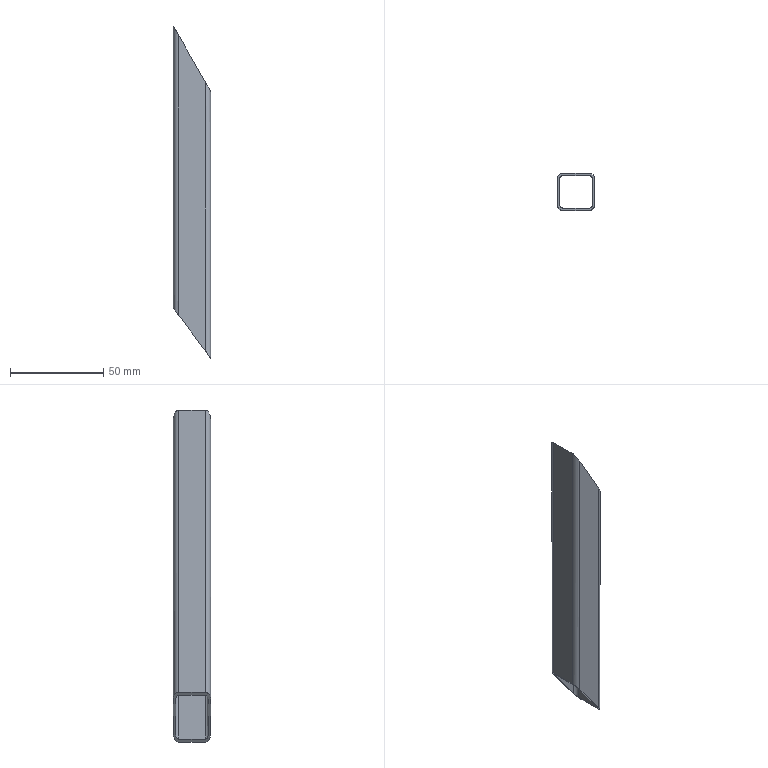Part | SolidWorks | features BaseBody 1 | 1 solid | 18 faces | box 20 x 20 x 178.33 mm | volume 12571 mm3 | plane 10 | cylinder 8 | commonest cylinder face diameters 3.6 x4 6 x4
STEP:
#1=CARTESIAN_POINT('',(-10.,-7.,172.164));
#2=VERTEX_POINT('',#1);
#3=CARTESIAN_POINT('',(-10.,7.,172.164));
#4=VERTEX_POINT('',#3);
#5=CARTESIAN_POINT('',(-10.,-7.,172.164));
#6=DIRECTION('',(0.,1.,0.));
#7=VECTOR('',#6,1000.);
#8=LINE('',#5,#7);
#9=EDGE_CURVE('',#2,#4,#8,.T.);
#10=ORIENTED_EDGE('',*,*,#9,.T.);
#11=CARTESIAN_POINT('',(-10.,7.,20.642));
#12=VERTEX_POINT('',#11);
#13=CARTESIAN_POINT('',(-10.,7.,0.));
#14=DIRECTION('',(0.,0.,-1.));
#15=VECTOR('',#14,1000.);
#16=LINE('',#13,#15);
#17=EDGE_CURVE('',#4,#12,#16,.T.);
#18=ORIENTED_EDGE('',*,*,#17,.T.);
#19=CARTESIAN_POINT('',(-10.,-7.,20.642));
#20=VERTEX_POINT('',#19);
#21=CARTESIAN_POINT('',(-10.,-7.,20.642));
#22=DIRECTION('',(0.,-1.,0.));
#23=VECTOR('',#22,1000.);
#24=LINE('',#21,#23);
#25=EDGE_CURVE('',#12,#20,#24,.T.);
#26=ORIENTED_EDGE('',*,*,#25,.T.);
#27=CARTESIAN_POINT('',(-10.,-7.,0.));
#28=DIRECTION('',(0.,0.,1.));
#29=VECTOR('',#28,1000.);
#30=LINE('',#27,#29);
#31=EDGE_CURVE('',#20,#2,#30,.T.);
#32=ORIENTED_EDGE('',*,*,#31,.T.);
#33=EDGE_LOOP('',(#10,#18,#26,#32));
#34=FACE_OUTER_BOUND('',#33,.T.);
#35=CARTESIAN_POINT('',(-10.,-7.,0.));
#36=DIRECTION('',(-1.,0.,0.));
#37=DIRECTION('',(0.,-1.,0.));
#38=AXIS2_PLACEMENT_3D('',#35,#36,#37);
#39=PLANE('',#38);
#40=ADVANCED_FACE('',(#34),#39,.T.);
#41=CARTESIAN_POINT('',(-7.,10.,166.9));
#42=VERTEX_POINT('',#41);
#43=CARTESIAN_POINT('',(-10.,7.,172.164));
#44=CARTESIAN_POINT('',(-10.,8.757,172.164));
#45=CARTESIAN_POINT('',(-8.757,10.,169.984));
#46=CARTESIAN_POINT('',(-7.,10.,166.9));
#47=(BOUNDED_CURVE()B_SPLINE_CURVE(3,(#43,#44,#45,#46),.UNSPECIFIED.,.F.,.F.)B_SPLINE_CURVE_WITH_KNOTS((4,4),(0.,1.571),.UNSPECIFIED.)CURVE()GEOMETRIC_REPRESENTATION_ITEM()RATIONAL_B_SPLINE_CURVE((1.,0.8047,0.8047,1.))REPRESENTATION_ITEM(''));
#48=EDGE_CURVE('',#4,#42,#47,.T.);
#49=ORIENTED_EDGE('',*,*,#48,.T.);
#50=CARTESIAN_POINT('',(-7.,10.,16.621));
#51=VERTEX_POINT('',#50);
#52=CARTESIAN_POINT('',(-7.,10.,0.));
#53=DIRECTION('',(0.,0.,-1.));
#54=VECTOR('',#53,1000.);
#55=LINE('',#52,#54);
#56=EDGE_CURVE('',#42,#51,#55,.T.);
#57=ORIENTED_EDGE('',*,*,#56,.T.);
#58=CARTESIAN_POINT('',(-7.,10.,16.621));
#59=CARTESIAN_POINT('',(-8.757,10.,18.976));
#60=CARTESIAN_POINT('',(-10.,8.757,20.642));
#61=CARTESIAN_POINT('',(-10.,7.,20.642));
#62=(BOUNDED_CURVE()B_SPLINE_CURVE(3,(#58,#59,#60,#61),.UNSPECIFIED.,.F.,.T.)B_SPLINE_CURVE_WITH_KNOTS((4,4),(4.712,6.283),.UNSPECIFIED.)CURVE()GEOMETRIC_REPRESENTATION_ITEM()RATIONAL_B_SPLINE_CURVE((1.,0.8047,0.8047,1.))REPRESENTATION_ITEM(''));
#63=EDGE_CURVE('',#51,#12,#62,.T.);
#64=ORIENTED_EDGE('',*,*,#63,.T.);
#65=ORIENTED_EDGE('',*,*,#17,.F.);
#66=EDGE_LOOP('',(#49,#57,#64,#65));
#67=FACE_OUTER_BOUND('',#66,.T.);
#68=CARTESIAN_POINT('',(-7.,7.,0.));
#69=DIRECTION('',(0.,0.,1.));
#70=DIRECTION('',(1.,0.,0.));
#71=AXIS2_PLACEMENT_3D('',#68,#69,#70);
#72=CYLINDRICAL_SURFACE('',#71,3.);
#73=ADVANCED_FACE('',(#67),#72,.T.);
#74=CARTESIAN_POINT('',(-8.8,-7.,170.059));
#75=VERTEX_POINT('',#74);
#76=CARTESIAN_POINT('',(-7.,-8.8,166.9));
#77=VERTEX_POINT('',#76);
#78=CARTESIAN_POINT('',(-8.8,-7.,170.059));
#79=CARTESIAN_POINT('',(-8.8,-8.054,170.059));
#80=CARTESIAN_POINT('',(-8.054,-8.8,168.75));
#81=CARTESIAN_POINT('',(-7.,-8.8,166.9));
#82=(BOUNDED_CURVE()B_SPLINE_CURVE(3,(#78,#79,#80,#81),.UNSPECIFIED.,.F.,.F.)B_SPLINE_CURVE_WITH_KNOTS((4,4),(0.,1.571),.UNSPECIFIED.)CURVE()GEOMETRIC_REPRESENTATION_ITEM()RATIONAL_B_SPLINE_CURVE((1.,0.8047,0.8047,1.))REPRESENTATION_ITEM(''));
#83=EDGE_CURVE('',#75,#77,#82,.T.);
#84=ORIENTED_EDGE('',*,*,#83,.F.);
#85=CARTESIAN_POINT('',(-8.8,7.,170.059));
#86=VERTEX_POINT('',#85);
#87=CARTESIAN_POINT('',(-8.8,0.,170.059));
#88=DIRECTION('',(0.,-1.,0.));
#89=VECTOR('',#88,1000.);
#90=LINE('',#87,#89);
#91=EDGE_CURVE('',#86,#75,#90,.T.);
#92=ORIENTED_EDGE('',*,*,#91,.F.);
#93=CARTESIAN_POINT('',(-7.,8.8,166.9));
#94=VERTEX_POINT('',#93);
#95=CARTESIAN_POINT('',(-7.,8.8,166.9));
#96=CARTESIAN_POINT('',(-8.054,8.8,168.75));
#97=CARTESIAN_POINT('',(-8.8,8.054,170.059));
#98=CARTESIAN_POINT('',(-8.8,7.,170.059));
#99=(BOUNDED_CURVE()B_SPLINE_CURVE(3,(#95,#96,#97,#98),.UNSPECIFIED.,.F.,.T.)B_SPLINE_CURVE_WITH_KNOTS((4,4),(4.712,6.283),.UNSPECIFIED.)CURVE()GEOMETRIC_REPRESENTATION_ITEM()RATIONAL_B_SPLINE_CURVE((1.,0.8047,0.8047,1.))REPRESENTATION_ITEM(''));
#100=EDGE_CURVE('',#94,#86,#99,.T.);
#101=ORIENTED_EDGE('',*,*,#100,.F.);
#102=CARTESIAN_POINT('',(7.,8.8,142.333));
#103=VERTEX_POINT('',#102);
#104=CARTESIAN_POINT('',(66.512,8.8,37.903));
#105=DIRECTION('',(-0.4951,0.,0.8688));
#106=VECTOR('',#105,1000.);
#107=LINE('',#104,#106);
#108=EDGE_CURVE('',#103,#94,#107,.T.);
#109=ORIENTED_EDGE('',*,*,#108,.F.);
#110=CARTESIAN_POINT('',(8.8,7.,139.174));
#111=VERTEX_POINT('',#110);
#112=CARTESIAN_POINT('',(8.8,7.,139.174));
#113=CARTESIAN_POINT('',(8.8,8.054,139.174));
#114=CARTESIAN_POINT('',(8.054,8.8,140.483));
#115=CARTESIAN_POINT('',(7.,8.8,142.333));
#116=(BOUNDED_CURVE()B_SPLINE_CURVE(3,(#112,#113,#114,#115),.UNSPECIFIED.,.F.,.T.)B_SPLINE_CURVE_WITH_KNOTS((4,4),(3.142,4.712),.UNSPECIFIED.)CURVE()GEOMETRIC_REPRESENTATION_ITEM()RATIONAL_B_SPLINE_CURVE((1.,0.8047,0.8047,1.))REPRESENTATION_ITEM(''));
#117=EDGE_CURVE('',#111,#103,#116,.T.);
#118=ORIENTED_EDGE('',*,*,#117,.F.);
#119=CARTESIAN_POINT('',(8.8,-7.,139.174));
#120=VERTEX_POINT('',#119);
#121=CARTESIAN_POINT('',(8.8,0.,139.174));
#122=DIRECTION('',(0.,1.,0.));
#123=VECTOR('',#122,1000.);
#124=LINE('',#121,#123);
#125=EDGE_CURVE('',#120,#111,#124,.T.);
#126=ORIENTED_EDGE('',*,*,#125,.F.);
#127=CARTESIAN_POINT('',(7.,-8.8,142.333));
#128=VERTEX_POINT('',#127);
#129=CARTESIAN_POINT('',(7.,-8.8,142.333));
#130=CARTESIAN_POINT('',(8.054,-8.8,140.483));
#131=CARTESIAN_POINT('',(8.8,-8.054,139.174));
#132=CARTESIAN_POINT('',(8.8,-7.,139.174));
#133=(BOUNDED_CURVE()B_SPLINE_CURVE(3,(#129,#130,#131,#132),.UNSPECIFIED.,.F.,.F.)B_SPLINE_CURVE_WITH_KNOTS((4,4),(1.571,3.142),.UNSPECIFIED.)CURVE()GEOMETRIC_REPRESENTATION_ITEM()RATIONAL_B_SPLINE_CURVE((1.,0.8047,0.8047,1.))REPRESENTATION_ITEM(''));
#134=EDGE_CURVE('',#128,#120,#133,.T.);
#135=ORIENTED_EDGE('',*,*,#134,.F.);
#136=CARTESIAN_POINT('',(66.512,-8.8,37.903));
#137=DIRECTION('',(0.4951,0.,-0.8688));
#138=VECTOR('',#137,1000.);
#139=LINE('',#136,#138);
#140=EDGE_CURVE('',#77,#128,#139,.T.);
#141=ORIENTED_EDGE('',*,*,#140,.F.);
#142=EDGE_LOOP('',(#84,#92,#101,#109,#118,#126,#135,#141));
#143=FACE_BOUND('',#142,.T.);
#144=CARTESIAN_POINT('',(7.,10.,142.333));
#145=VERTEX_POINT('',#144);
#146=CARTESIAN_POINT('',(10.,7.,137.069));
#147=VERTEX_POINT('',#146);
#148=CARTESIAN_POINT('',(7.,10.,142.333));
#149=CARTESIAN_POINT('',(8.757,10.,139.249));
#150=CARTESIAN_POINT('',(10.,8.757,137.069));
#151=CARTESIAN_POINT('',(10.,7.,137.069));
#152=(BOUNDED_CURVE()B_SPLINE_CURVE(3,(#148,#149,#150,#151),.UNSPECIFIED.,.F.,.F.)B_SPLINE_CURVE_WITH_KNOTS((4,4),(1.571,3.142),.UNSPECIFIED.)CURVE()GEOMETRIC_REPRESENTATION_ITEM()RATIONAL_B_SPLINE_CURVE((1.,0.8047,0.8047,1.))REPRESENTATION_ITEM(''));
#153=EDGE_CURVE('',#145,#147,#152,.T.);
#154=ORIENTED_EDGE('',*,*,#153,.F.);
#155=CARTESIAN_POINT('',(66.512,10.,37.903));
#156=DIRECTION('',(0.4951,0.,-0.8688));
#157=VECTOR('',#156,1000.);
#158=LINE('',#155,#157);
#159=EDGE_CURVE('',#42,#145,#158,.T.);
#160=ORIENTED_EDGE('',*,*,#159,.F.);
#161=ORIENTED_EDGE('',*,*,#48,.F.);
#162=ORIENTED_EDGE('',*,*,#9,.F.);
#163=CARTESIAN_POINT('',(-7.,-10.,166.9));
#164=VERTEX_POINT('',#163);
#165=CARTESIAN_POINT('',(-7.,-10.,166.9));
#166=CARTESIAN_POINT('',(-8.757,-10.,169.984));
#167=CARTESIAN_POINT('',(-10.,-8.757,172.164));
#168=CARTESIAN_POINT('',(-10.,-7.,172.164));
#169=(BOUNDED_CURVE()B_SPLINE_CURVE(3,(#165,#166,#167,#168),.UNSPECIFIED.,.F.,.F.)B_SPLINE_CURVE_WITH_KNOTS((4,4),(4.712,6.283),.UNSPECIFIED.)CURVE()GEOMETRIC_REPRESENTATION_ITEM()RATIONAL_B_SPLINE_CURVE((1.,0.8047,0.8047,1.))REPRESENTATION_ITEM(''));
#170=EDGE_CURVE('',#164,#2,#169,.T.);
#171=ORIENTED_EDGE('',*,*,#170,.F.);
#172=CARTESIAN_POINT('',(7.,-10.,142.333));
#173=VERTEX_POINT('',#172);
#174=CARTESIAN_POINT('',(66.512,-10.,37.903));
#175=DIRECTION('',(-0.4951,0.,0.8688));
#176=VECTOR('',#175,1000.);
#177=LINE('',#174,#176);
#178=EDGE_CURVE('',#173,#164,#177,.T.);
#179=ORIENTED_EDGE('',*,*,#178,.F.);
#180=CARTESIAN_POINT('',(10.,-7.,137.069));
#181=VERTEX_POINT('',#180);
#182=CARTESIAN_POINT('',(10.,-7.,137.069));
#183=CARTESIAN_POINT('',(10.,-8.757,137.069));
#184=CARTESIAN_POINT('',(8.757,-10.,139.249));
#185=CARTESIAN_POINT('',(7.,-10.,142.333));
#186=(BOUNDED_CURVE()B_SPLINE_CURVE(3,(#182,#183,#184,#185),.UNSPECIFIED.,.F.,.F.)B_SPLINE_CURVE_WITH_KNOTS((4,4),(3.142,4.712),.UNSPECIFIED.)CURVE()GEOMETRIC_REPRESENTATION_ITEM()RATIONAL_B_SPLINE_CURVE((1.,0.8047,0.8047,1.))REPRESENTATION_ITEM(''));
#187=EDGE_CURVE('',#181,#173,#186,.T.);
#188=ORIENTED_EDGE('',*,*,#187,.F.);
#189=CARTESIAN_POINT('',(10.,0.,137.069));
#190=DIRECTION('',(0.,-1.,0.));
#191=VECTOR('',#190,1000.);
#192=LINE('',#189,#191);
#193=EDGE_CURVE('',#147,#181,#192,.T.);
#194=ORIENTED_EDGE('',*,*,#193,.F.);
#195=EDGE_LOOP('',(#154,#160,#161,#162,#171,#179,#188,#194));
#196=FACE_OUTER_BOUND('',#195,.T.);
#197=CARTESIAN_POINT('',(66.512,0.,37.903));
#198=DIRECTION('',(-0.8688,0.,-0.4951));
#199=DIRECTION('',(-0.4951,0.,0.8688));
#200=AXIS2_PLACEMENT_3D('',#197,#198,#199);
#201=PLANE('',#200);
#202=ADVANCED_FACE('',(#143,#196),#201,.F.);
#203=ORIENTED_EDGE('',*,*,#170,.T.);
#204=ORIENTED_EDGE('',*,*,#31,.F.);
#205=CARTESIAN_POINT('',(-7.,-10.,16.621));
#206=VERTEX_POINT('',#205);
#207=CARTESIAN_POINT('',(-10.,-7.,20.642));
#208=CARTESIAN_POINT('',(-10.,-8.757,20.642));
#209=CARTESIAN_POINT('',(-8.757,-10.,18.976));
#210=CARTESIAN_POINT('',(-7.,-10.,16.621));
#211=(BOUNDED_CURVE()B_SPLINE_CURVE(3,(#207,#208,#209,#210),.UNSPECIFIED.,.F.,.F.)B_SPLINE_CURVE_WITH_KNOTS((4,4),(0.,1.571),.UNSPECIFIED.)CURVE()GEOMETRIC_REPRESENTATION_ITEM()RATIONAL_B_SPLINE_CURVE((1.,0.8047,0.8047,1.))REPRESENTATION_ITEM(''));
#212=EDGE_CURVE('',#20,#206,#211,.T.);
#213=ORIENTED_EDGE('',*,*,#212,.T.);
#214=CARTESIAN_POINT('',(-7.,-10.,0.));
#215=DIRECTION('',(0.,0.,1.));
#216=VECTOR('',#215,1000.);
#217=LINE('',#214,#216);
#218=EDGE_CURVE('',#206,#164,#217,.T.);
#219=ORIENTED_EDGE('',*,*,#218,.T.);
#220=EDGE_LOOP('',(#203,#204,#213,#219));
#221=FACE_OUTER_BOUND('',#220,.T.);
#222=CARTESIAN_POINT('',(-7.,-7.,0.));
#223=DIRECTION('',(0.,0.,1.));
#224=DIRECTION('',(1.,0.,0.));
#225=AXIS2_PLACEMENT_3D('',#222,#223,#224);
#226=CYLINDRICAL_SURFACE('',#225,3.);
#227=ADVANCED_FACE('',(#221),#226,.T.);
#228=CARTESIAN_POINT('',(-8.8,7.,19.034));
#229=VERTEX_POINT('',#228);
#230=CARTESIAN_POINT('',(-7.,8.8,16.621));
#231=VERTEX_POINT('',#230);
#232=CARTESIAN_POINT('',(-8.8,7.,19.034));
#233=CARTESIAN_POINT('',(-8.8,8.054,19.034));
#234=CARTESIAN_POINT('',(-8.054,8.8,18.034));
#235=CARTESIAN_POINT('',(-7.,8.8,16.621));
#236=(BOUNDED_CURVE()B_SPLINE_CURVE(3,(#232,#233,#234,#235),.UNSPECIFIED.,.F.,.F.)B_SPLINE_CURVE_WITH_KNOTS((4,4),(0.,1.571),.UNSPECIFIED.)CURVE()GEOMETRIC_REPRESENTATION_ITEM()RATIONAL_B_SPLINE_CURVE((1.,0.8047,0.8047,1.))REPRESENTATION_ITEM(''));
#237=EDGE_CURVE('',#229,#231,#236,.T.);
#238=ORIENTED_EDGE('',*,*,#237,.F.);
#239=CARTESIAN_POINT('',(-8.8,-7.,19.034));
#240=VERTEX_POINT('',#239);
#241=CARTESIAN_POINT('',(-8.8,0.,19.034));
#242=DIRECTION('',(0.,1.,0.));
#243=VECTOR('',#242,1000.);
#244=LINE('',#241,#243);
#245=EDGE_CURVE('',#240,#229,#244,.T.);
#246=ORIENTED_EDGE('',*,*,#245,.F.);
#247=CARTESIAN_POINT('',(-7.,-8.8,16.621));
#248=VERTEX_POINT('',#247);
#249=CARTESIAN_POINT('',(-7.,-8.8,16.621));
#250=CARTESIAN_POINT('',(-8.054,-8.8,18.034));
#251=CARTESIAN_POINT('',(-8.8,-8.054,19.034));
#252=CARTESIAN_POINT('',(-8.8,-7.,19.034));
#253=(BOUNDED_CURVE()B_SPLINE_CURVE(3,(#249,#250,#251,#252),.UNSPECIFIED.,.F.,.F.)B_SPLINE_CURVE_WITH_KNOTS((4,4),(4.712,6.283),.UNSPECIFIED.)CURVE()GEOMETRIC_REPRESENTATION_ITEM()RATIONAL_B_SPLINE_CURVE((1.,0.8047,0.8047,1.))REPRESENTATION_ITEM(''));
#254=EDGE_CURVE('',#248,#240,#253,.T.);
#255=ORIENTED_EDGE('',*,*,#254,.F.);
#256=CARTESIAN_POINT('',(7.,-8.8,-2.144));
#257=VERTEX_POINT('',#256);
#258=CARTESIAN_POINT('',(3.469,-8.8,2.588));
#259=DIRECTION('',(-0.598,0.,0.8015));
#260=VECTOR('',#259,1000.);
#261=LINE('',#258,#260);
#262=EDGE_CURVE('',#257,#248,#261,.T.);
#263=ORIENTED_EDGE('',*,*,#262,.F.);
#264=CARTESIAN_POINT('',(8.8,-7.,-4.557));
#265=VERTEX_POINT('',#264);
#266=CARTESIAN_POINT('',(8.8,-7.,-4.557));
#267=CARTESIAN_POINT('',(8.8,-8.054,-4.557));
#268=CARTESIAN_POINT('',(8.054,-8.8,-3.557));
#269=CARTESIAN_POINT('',(7.,-8.8,-2.144));
#270=(BOUNDED_CURVE()B_SPLINE_CURVE(3,(#266,#267,#268,#269),.UNSPECIFIED.,.F.,.F.)B_SPLINE_CURVE_WITH_KNOTS((4,4),(3.142,4.712),.UNSPECIFIED.)CURVE()GEOMETRIC_REPRESENTATION_ITEM()RATIONAL_B_SPLINE_CURVE((1.,0.8047,0.8047,1.))REPRESENTATION_ITEM(''));
#271=EDGE_CURVE('',#265,#257,#270,.T.);
#272=ORIENTED_EDGE('',*,*,#271,.F.);
#273=CARTESIAN_POINT('',(8.8,7.,-4.557));
#274=VERTEX_POINT('',#273);
#275=CARTESIAN_POINT('',(8.8,0.,-4.557));
#276=DIRECTION('',(0.,-1.,0.));
#277=VECTOR('',#276,1000.);
#278=LINE('',#275,#277);
#279=EDGE_CURVE('',#274,#265,#278,.T.);
#280=ORIENTED_EDGE('',*,*,#279,.F.);
#281=CARTESIAN_POINT('',(7.,8.8,-2.144));
#282=VERTEX_POINT('',#281);
#283=CARTESIAN_POINT('',(7.,8.8,-2.144));
#284=CARTESIAN_POINT('',(8.054,8.8,-3.557));
#285=CARTESIAN_POINT('',(8.8,8.054,-4.557));
#286=CARTESIAN_POINT('',(8.8,7.,-4.557));
#287=(BOUNDED_CURVE()B_SPLINE_CURVE(3,(#283,#284,#285,#286),.UNSPECIFIED.,.F.,.F.)B_SPLINE_CURVE_WITH_KNOTS((4,4),(1.571,3.142),.UNSPECIFIED.)CURVE()GEOMETRIC_REPRESENTATION_ITEM()RATIONAL_B_SPLINE_CURVE((1.,0.8047,0.8047,1.))REPRESENTATION_ITEM(''));
#288=EDGE_CURVE('',#282,#274,#287,.T.);
#289=ORIENTED_EDGE('',*,*,#288,.F.);
#290=CARTESIAN_POINT('',(3.469,8.8,2.588));
#291=DIRECTION('',(0.598,0.,-0.8015));
#292=VECTOR('',#291,1000.);
#293=LINE('',#290,#292);
#294=EDGE_CURVE('',#231,#282,#293,.T.);
#295=ORIENTED_EDGE('',*,*,#294,.F.);
#296=EDGE_LOOP('',(#238,#246,#255,#263,#272,#280,#289,#295));
#297=FACE_BOUND('',#296,.T.);
#298=CARTESIAN_POINT('',(7.,10.,-2.144));
#299=VERTEX_POINT('',#298);
#300=CARTESIAN_POINT('',(3.469,10.,2.588));
#301=DIRECTION('',(-0.598,0.,0.8015));
#302=VECTOR('',#301,1000.);
#303=LINE('',#300,#302);
#304=EDGE_CURVE('',#299,#51,#303,.T.);
#305=ORIENTED_EDGE('',*,*,#304,.F.);
#306=CARTESIAN_POINT('',(10.,7.,-6.165));
#307=VERTEX_POINT('',#306);
#308=CARTESIAN_POINT('',(10.,7.,-6.165));
#309=CARTESIAN_POINT('',(10.,8.757,-6.165));
#310=CARTESIAN_POINT('',(8.757,10.,-4.5));
#311=CARTESIAN_POINT('',(7.,10.,-2.144));
#312=(BOUNDED_CURVE()B_SPLINE_CURVE(3,(#308,#309,#310,#311),.UNSPECIFIED.,.F.,.F.)B_SPLINE_CURVE_WITH_KNOTS((4,4),(3.142,4.712),.UNSPECIFIED.)CURVE()GEOMETRIC_REPRESENTATION_ITEM()RATIONAL_B_SPLINE_CURVE((1.,0.8047,0.8047,1.))REPRESENTATION_ITEM(''));
#313=EDGE_CURVE('',#307,#299,#312,.T.);
#314=ORIENTED_EDGE('',*,*,#313,.F.);
#315=CARTESIAN_POINT('',(10.,-7.,-6.165));
#316=VERTEX_POINT('',#315);
#317=CARTESIAN_POINT('',(10.,0.,-6.165));
#318=DIRECTION('',(0.,1.,0.));
#319=VECTOR('',#318,1000.);
#320=LINE('',#317,#319);
#321=EDGE_CURVE('',#316,#307,#320,.T.);
#322=ORIENTED_EDGE('',*,*,#321,.F.);
#323=CARTESIAN_POINT('',(7.,-10.,-2.144));
#324=VERTEX_POINT('',#323);
#325=CARTESIAN_POINT('',(7.,-10.,-2.144));
#326=CARTESIAN_POINT('',(8.757,-10.,-4.5));
#327=CARTESIAN_POINT('',(10.,-8.757,-6.165));
#328=CARTESIAN_POINT('',(10.,-7.,-6.165));
#329=(BOUNDED_CURVE()B_SPLINE_CURVE(3,(#325,#326,#327,#328),.UNSPECIFIED.,.F.,.F.)B_SPLINE_CURVE_WITH_KNOTS((4,4),(1.571,3.142),.UNSPECIFIED.)CURVE()GEOMETRIC_REPRESENTATION_ITEM()RATIONAL_B_SPLINE_CURVE((1.,0.8047,0.8047,1.))REPRESENTATION_ITEM(''));
#330=EDGE_CURVE('',#324,#316,#329,.T.);
#331=ORIENTED_EDGE('',*,*,#330,.F.);
#332=CARTESIAN_POINT('',(3.469,-10.,2.588));
#333=DIRECTION('',(0.598,0.,-0.8015));
#334=VECTOR('',#333,1000.);
#335=LINE('',#332,#334);
#336=EDGE_CURVE('',#206,#324,#335,.T.);
#337=ORIENTED_EDGE('',*,*,#336,.F.);
#338=ORIENTED_EDGE('',*,*,#212,.F.);
#339=ORIENTED_EDGE('',*,*,#25,.F.);
#340=ORIENTED_EDGE('',*,*,#63,.F.);
#341=EDGE_LOOP('',(#305,#314,#322,#331,#337,#338,#339,#340));
#342=FACE_OUTER_BOUND('',#341,.T.);
#343=CARTESIAN_POINT('',(3.469,0.,2.588));
#344=DIRECTION('',(0.8015,0.,0.598));
#345=DIRECTION('',(0.598,0.,-0.8015));
#346=AXIS2_PLACEMENT_3D('',#343,#344,#345);
#347=PLANE('',#346);
#348=ADVANCED_FACE('',(#297,#342),#347,.F.);
#349=ORIENTED_EDGE('',*,*,#159,.T.);
#350=CARTESIAN_POINT('',(7.,10.,0.));
#351=DIRECTION('',(0.,0.,-1.));
#352=VECTOR('',#351,1000.);
#353=LINE('',#350,#352);
#354=EDGE_CURVE('',#145,#299,#353,.T.);
#355=ORIENTED_EDGE('',*,*,#354,.T.);
#356=ORIENTED_EDGE('',*,*,#304,.T.);
#357=ORIENTED_EDGE('',*,*,#56,.F.);
#358=EDGE_LOOP('',(#349,#355,#356,#357));
#359=FACE_OUTER_BOUND('',#358,.T.);
#360=CARTESIAN_POINT('',(-7.,10.,0.));
#361=DIRECTION('',(0.,1.,0.));
#362=DIRECTION('',(-1.,0.,0.));
#363=AXIS2_PLACEMENT_3D('',#360,#361,#362);
#364=PLANE('',#363);
#365=ADVANCED_FACE('',(#359),#364,.T.);
#366=CARTESIAN_POINT('',(-7.,-8.8,0.));
#367=DIRECTION('',(0.,0.,-1.));
#368=VECTOR('',#367,1000.);
#369=LINE('',#366,#368);
#370=EDGE_CURVE('',#77,#248,#369,.T.);
#371=ORIENTED_EDGE('',*,*,#370,.F.);
#372=ORIENTED_EDGE('',*,*,#140,.T.);
#373=CARTESIAN_POINT('',(7.,-8.8,0.));
#374=DIRECTION('',(0.,0.,1.));
#375=VECTOR('',#374,1000.);
#376=LINE('',#373,#375);
#377=EDGE_CURVE('',#257,#128,#376,.T.);
#378=ORIENTED_EDGE('',*,*,#377,.F.);
#379=ORIENTED_EDGE('',*,*,#262,.T.);
#380=EDGE_LOOP('',(#371,#372,#378,#379));
#381=FACE_OUTER_BOUND('',#380,.T.);
#382=CARTESIAN_POINT('',(7.,-8.8,0.));
#383=DIRECTION('',(0.,-1.,0.));
#384=DIRECTION('',(1.,0.,0.));
#385=AXIS2_PLACEMENT_3D('',#382,#383,#384);
#386=PLANE('',#385);
#387=ADVANCED_FACE('',(#381),#386,.F.);
#388=CARTESIAN_POINT('',(-8.8,-7.,0.));
#389=DIRECTION('',(0.,0.,-1.));
#390=VECTOR('',#389,1000.);
#391=LINE('',#388,#390);
#392=EDGE_CURVE('',#75,#240,#391,.T.);
#393=ORIENTED_EDGE('',*,*,#392,.F.);
#394=ORIENTED_EDGE('',*,*,#83,.T.);
#395=ORIENTED_EDGE('',*,*,#370,.T.);
#396=ORIENTED_EDGE('',*,*,#254,.T.);
#397=EDGE_LOOP('',(#393,#394,#395,#396));
#398=FACE_OUTER_BOUND('',#397,.T.);
#399=CARTESIAN_POINT('',(-7.,-7.,0.));
#400=DIRECTION('',(0.,0.,1.));
#401=DIRECTION('',(1.,0.,0.));
#402=AXIS2_PLACEMENT_3D('',#399,#400,#401);
#403=CYLINDRICAL_SURFACE('',#402,1.8);
#404=ADVANCED_FACE('',(#398),#403,.F.);
#405=CARTESIAN_POINT('',(-8.8,7.,0.));
#406=DIRECTION('',(0.,0.,-1.));
#407=VECTOR('',#406,1000.);
#408=LINE('',#405,#407);
#409=EDGE_CURVE('',#86,#229,#408,.T.);
#410=ORIENTED_EDGE('',*,*,#409,.F.);
#411=ORIENTED_EDGE('',*,*,#91,.T.);
#412=ORIENTED_EDGE('',*,*,#392,.T.);
#413=ORIENTED_EDGE('',*,*,#245,.T.);
#414=EDGE_LOOP('',(#410,#411,#412,#413));
#415=FACE_OUTER_BOUND('',#414,.T.);
#416=CARTESIAN_POINT('',(-8.8,-7.,0.));
#417=DIRECTION('',(-1.,0.,0.));
#418=DIRECTION('',(0.,-1.,0.));
#419=AXIS2_PLACEMENT_3D('',#416,#417,#418);
#420=PLANE('',#419);
#421=ADVANCED_FACE('',(#415),#420,.F.);
#422=CARTESIAN_POINT('',(-7.,8.8,0.));
#423=DIRECTION('',(0.,0.,-1.));
#424=VECTOR('',#423,1000.);
#425=LINE('',#422,#424);
#426=EDGE_CURVE('',#94,#231,#425,.T.);
#427=ORIENTED_EDGE('',*,*,#426,.F.);
#428=ORIENTED_EDGE('',*,*,#100,.T.);
#429=ORIENTED_EDGE('',*,*,#409,.T.);
#430=ORIENTED_EDGE('',*,*,#237,.T.);
#431=EDGE_LOOP('',(#427,#428,#429,#430));
#432=FACE_OUTER_BOUND('',#431,.T.);
#433=CARTESIAN_POINT('',(-7.,7.,0.));
#434=DIRECTION('',(0.,0.,1.));
#435=DIRECTION('',(1.,0.,0.));
#436=AXIS2_PLACEMENT_3D('',#433,#434,#435);
#437=CYLINDRICAL_SURFACE('',#436,1.8);
#438=ADVANCED_FACE('',(#432),#437,.F.);
#439=CARTESIAN_POINT('',(7.,8.8,0.));
#440=DIRECTION('',(0.,0.,-1.));
#441=VECTOR('',#440,1000.);
#442=LINE('',#439,#441);
#443=EDGE_CURVE('',#103,#282,#442,.T.);
#444=ORIENTED_EDGE('',*,*,#443,.F.);
#445=ORIENTED_EDGE('',*,*,#108,.T.);
#446=ORIENTED_EDGE('',*,*,#426,.T.);
#447=ORIENTED_EDGE('',*,*,#294,.T.);
#448=EDGE_LOOP('',(#444,#445,#446,#447));
#449=FACE_OUTER_BOUND('',#448,.T.);
#450=CARTESIAN_POINT('',(-7.,8.8,0.));
#451=DIRECTION('',(0.,1.,0.));
#452=DIRECTION('',(-1.,0.,0.));
#453=AXIS2_PLACEMENT_3D('',#450,#451,#452);
#454=PLANE('',#453);
#455=ADVANCED_FACE('',(#449),#454,.F.);
#456=CARTESIAN_POINT('',(8.8,7.,0.));
#457=DIRECTION('',(0.,0.,-1.));
#458=VECTOR('',#457,1000.);
#459=LINE('',#456,#458);
#460=EDGE_CURVE('',#111,#274,#459,.T.);
#461=ORIENTED_EDGE('',*,*,#460,.F.);
#462=ORIENTED_EDGE('',*,*,#117,.T.);
#463=ORIENTED_EDGE('',*,*,#443,.T.);
#464=ORIENTED_EDGE('',*,*,#288,.T.);
#465=EDGE_LOOP('',(#461,#462,#463,#464));
#466=FACE_OUTER_BOUND('',#465,.T.);
#467=CARTESIAN_POINT('',(7.,7.,0.));
#468=DIRECTION('',(0.,0.,1.));
#469=DIRECTION('',(1.,0.,0.));
#470=AXIS2_PLACEMENT_3D('',#467,#468,#469);
#471=CYLINDRICAL_SURFACE('',#470,1.8);
#472=ADVANCED_FACE('',(#466),#471,.F.);
#473=CARTESIAN_POINT('',(8.8,-7.,0.));
#474=DIRECTION('',(0.,0.,-1.));
#475=VECTOR('',#474,1000.);
#476=LINE('',#473,#475);
#477=EDGE_CURVE('',#120,#265,#476,.T.);
#478=ORIENTED_EDGE('',*,*,#477,.F.);
#479=ORIENTED_EDGE('',*,*,#125,.T.);
#480=ORIENTED_EDGE('',*,*,#460,.T.);
#481=ORIENTED_EDGE('',*,*,#279,.T.);
#482=EDGE_LOOP('',(#478,#479,#480,#481));
#483=FACE_OUTER_BOUND('',#482,.T.);
#484=CARTESIAN_POINT('',(8.8,7.,0.));
#485=DIRECTION('',(1.,0.,0.));
#486=DIRECTION('',(0.,0.,-1.));
#487=AXIS2_PLACEMENT_3D('',#484,#485,#486);
#488=PLANE('',#487);
#489=ADVANCED_FACE('',(#483),#488,.F.);
#490=ORIENTED_EDGE('',*,*,#377,.T.);
#491=ORIENTED_EDGE('',*,*,#134,.T.);
#492=ORIENTED_EDGE('',*,*,#477,.T.);
#493=ORIENTED_EDGE('',*,*,#271,.T.);
#494=EDGE_LOOP('',(#490,#491,#492,#493));
#495=FACE_OUTER_BOUND('',#494,.T.);
#496=CARTESIAN_POINT('',(7.,-7.,0.));
#497=DIRECTION('',(0.,0.,1.));
#498=DIRECTION('',(1.,0.,0.));
#499=AXIS2_PLACEMENT_3D('',#496,#497,#498);
#500=CYLINDRICAL_SURFACE('',#499,1.8);
#501=ADVANCED_FACE('',(#495),#500,.F.);
#502=ORIENTED_EDGE('',*,*,#321,.T.);
#503=CARTESIAN_POINT('',(10.,7.,0.));
#504=DIRECTION('',(0.,0.,1.));
#505=VECTOR('',#504,1000.);
#506=LINE('',#503,#505);
#507=EDGE_CURVE('',#307,#147,#506,.T.);
#508=ORIENTED_EDGE('',*,*,#507,.T.);
#509=ORIENTED_EDGE('',*,*,#193,.T.);
#510=CARTESIAN_POINT('',(10.,-7.,0.));
#511=DIRECTION('',(0.,0.,-1.));
#512=VECTOR('',#511,1000.);
#513=LINE('',#510,#512);
#514=EDGE_CURVE('',#181,#316,#513,.T.);
#515=ORIENTED_EDGE('',*,*,#514,.T.);
#516=EDGE_LOOP('',(#502,#508,#509,#515));
#517=FACE_OUTER_BOUND('',#516,.T.);
#518=CARTESIAN_POINT('',(10.,7.,0.));
#519=DIRECTION('',(1.,0.,0.));
#520=DIRECTION('',(0.,0.,-1.));
#521=AXIS2_PLACEMENT_3D('',#518,#519,#520);
#522=PLANE('',#521);
#523=ADVANCED_FACE('',(#517),#522,.T.);
#524=ORIENTED_EDGE('',*,*,#153,.T.);
#525=ORIENTED_EDGE('',*,*,#507,.F.);
#526=ORIENTED_EDGE('',*,*,#313,.T.);
#527=ORIENTED_EDGE('',*,*,#354,.F.);
#528=EDGE_LOOP('',(#524,#525,#526,#527));
#529=FACE_OUTER_BOUND('',#528,.T.);
#530=CARTESIAN_POINT('',(7.,7.,0.));
#531=DIRECTION('',(0.,0.,1.));
#532=DIRECTION('',(1.,0.,0.));
#533=AXIS2_PLACEMENT_3D('',#530,#531,#532);
#534=CYLINDRICAL_SURFACE('',#533,3.);
#535=ADVANCED_FACE('',(#529),#534,.T.);
#536=ORIENTED_EDGE('',*,*,#178,.T.);
#537=ORIENTED_EDGE('',*,*,#218,.F.);
#538=ORIENTED_EDGE('',*,*,#336,.T.);
#539=CARTESIAN_POINT('',(7.,-10.,0.));
#540=DIRECTION('',(0.,0.,1.));
#541=VECTOR('',#540,1000.);
#542=LINE('',#539,#541);
#543=EDGE_CURVE('',#324,#173,#542,.T.);
#544=ORIENTED_EDGE('',*,*,#543,.T.);
#545=EDGE_LOOP('',(#536,#537,#538,#544));
#546=FACE_OUTER_BOUND('',#545,.T.);
#547=CARTESIAN_POINT('',(7.,-10.,0.));
#548=DIRECTION('',(0.,-1.,0.));
#549=DIRECTION('',(1.,0.,0.));
#550=AXIS2_PLACEMENT_3D('',#547,#548,#549);
#551=PLANE('',#550);
#552=ADVANCED_FACE('',(#546),#551,.T.);
#553=ORIENTED_EDGE('',*,*,#187,.T.);
#554=ORIENTED_EDGE('',*,*,#543,.F.);
#555=ORIENTED_EDGE('',*,*,#330,.T.);
#556=ORIENTED_EDGE('',*,*,#514,.F.);
#557=EDGE_LOOP('',(#553,#554,#555,#556));
#558=FACE_OUTER_BOUND('',#557,.T.);
#559=CARTESIAN_POINT('',(7.,-7.,0.));
#560=DIRECTION('',(0.,0.,1.));
#561=DIRECTION('',(1.,0.,0.));
#562=AXIS2_PLACEMENT_3D('',#559,#560,#561);
#563=CYLINDRICAL_SURFACE('',#562,3.);
#564=ADVANCED_FACE('',(#558),#563,.T.);
#565=CLOSED_SHELL('',(#40,#73,#202,#227,#348,#365,#387,#404,#421,#438,#455,#472,#489,#501,#523,#535,#552,#564));
#566=MANIFOLD_SOLID_BREP('',#565);
#567=CARTESIAN_POINT('',(0.,0.,0.));
#568=DIRECTION('',(0.,0.,1.));
#569=DIRECTION('',(1.,0.,0.));
#570=AXIS2_PLACEMENT_3D('',#567,#568,#569);
#571=(LENGTH_UNIT()NAMED_UNIT(*)SI_UNIT(.MILLI.,.METRE.));
#572=UNCERTAINTY_MEASURE_WITH_UNIT(LENGTH_MEASURE(0.00001),#571,'','');
#573=(NAMED_UNIT(*)PLANE_ANGLE_UNIT()SI_UNIT($,.RADIAN.));
#574=(NAMED_UNIT(*)SI_UNIT($,.STERADIAN.)SOLID_ANGLE_UNIT());
#575=(GEOMETRIC_REPRESENTATION_CONTEXT(3)GLOBAL_UNCERTAINTY_ASSIGNED_CONTEXT((#572))GLOBAL_UNIT_ASSIGNED_CONTEXT((#571,#573,#574))REPRESENTATION_CONTEXT('',''));
#576=ADVANCED_BREP_SHAPE_REPRESENTATION('',(#566,#570),#575);